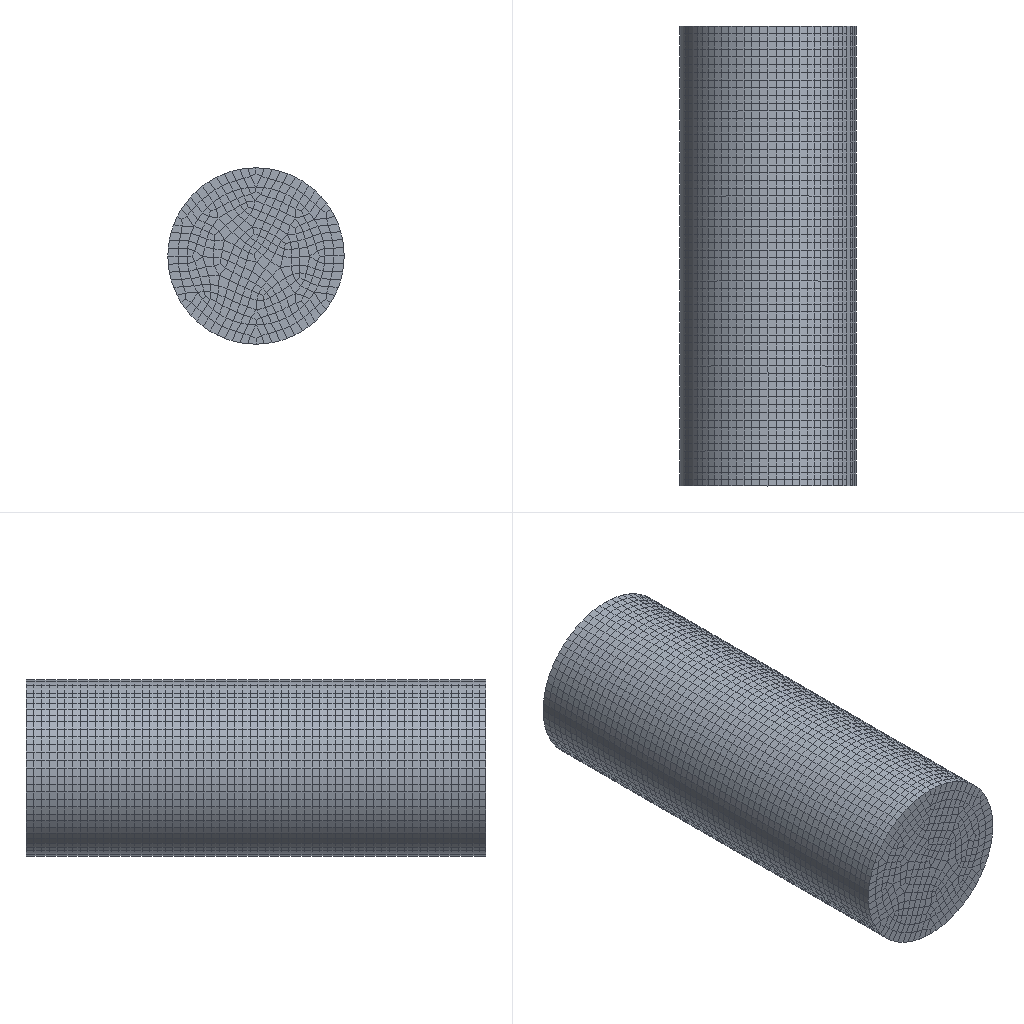Simulation study | ansys workbench
Ansys APDL input file, long lists of numbers shortened:
/batch
/config,noeldb,1     ! force off writing results to database
*get,_wallstrt,active,,time,wall
! ANSYS input file written by Workbench version 2020 R2
! File used for geometry attach:
/title,unsaved_project--___ (B5)
*DIM,_wb_ProjectScratch_dir,string,248
_wb_ProjectScratch_dir(1) = ''
*DIM,_wb_SolverFiles_dir,string,248
_wb_SolverFiles_dir(1) = ''
*DIM,_wb_userfiles_dir,string,248
_wb_userfiles_dir(1) = ''
/com,--- Data in consistent MKS units. See Solving Units in the help system for more information.
/units,MKS
/nopr
/wb,file,start              !  signify a WB generated input file
/prep7
! Turn off shape checking because checks already performed inside WB mesher.
! See help system for more information.
SHPP,OFF,,NOWARN
/nolist
etcon,set             ! allow ANSYS to choose best KEYOP's for 180x elements
/com,*********** Nodes for the whole assembly ***********
nblock,3,,50740
(1i9,3e20.9e3)
        1    -1.192148224E-02     0.000000000E+00    -1.104059469E-02
! (46127 more lines like these left out)
-1
/wb,elem,start            !  set before creation of elements
/com,*********** Elements for Body 1 "SYS\__" ***********
et,1,90
eblock,19,solid,,8511
(19i9)
        1        1        1        1        0        0        0        0       20        0        1      424      532    12288    12285      422      531    12424    12421
! (17021 more lines like these left out)
-1
/wb,elem,end               !  done creating elements
/com,*********** Send User Defined Coordinate System(s) ***********
csys,0
toffst,273.15,  ! Temperature offset from absolute zero
/wb,mat,start              !  starting to send materials
/com,*********** Send Materials ***********
Temperature = 'TEMP' ! Temperature
MP,DENS,1,7850,	! kg m^-3
MP,ALPX,1,1.2e-05,	! C^-1
MP,C,1,434,	! J kg^-1 C^-1
MP,KXX,1,60.5,	! W m^-1 C^-1
MP,RSVX,1,1.7e-07,	! kg m^3 A^-2 s^-3
MP,EX,1,200000000000,	! Pa
MP,NUXY,1,0.3,
MP,MURX,1,10000,
/wb,mat,end                !  done sending materials
!************************* Model Summary ********************
!SYS\__,	Structural Steel,	matid,	1
!************************* End Model Summary ********************
! get the diagonal of the bounding box. Needed later for other things
*get,_xmin,node,,mnloc,x
*get,_ymin,node,,mnloc,y
*get,_zmin,node,,mnloc,z
*get,_xmax,node,,mxloc,x
*get,_ymax,node,,mxloc,y
*get,_zmax,node,,mxloc,z
_ASMDIAG=(_xmax-_xmin)*(_xmax-_xmin)+(_ymax-_ymin)*(_ymax-_ymin)+(_zmax-_zmin)*(_zmax-_zmin)
_ASMDIAG=SQRT(_ASMDIAG)
/wb,contact,start          !  starting to send contact
/wb,contact,end            !  done creating contacts
/golist
/wb,load,start             !  starting to send loads
/com,*********** Define Temperature Constraint ***********
CMBLOCK,_CM52   ,NODE,    10344
(8i10)
       799       800       801       802       803       804       805       806
! (1292 more lines like these left out)
*DIM,_loadvari52,TABLE,2,1,1,TIME,
! Time values
_loadvari52(1,0,1) = 0.
_loadvari52(2,0,1) = 1.
! Load values
_loadvari52(1,1,1) = 100.
_loadvari52(2,1,1) = 100.
fcum,add                   ! add nodal forces up (needed in case have loads on the same edge,vertex)
fcum                       ! reset default on fcum command since done sending WB F loads
/com,*********** Create "______" ***********
et,2,152
eblock,10,,,4080
(15i9)
    16518        2        2        2        0    12215    12217    12081    12079    45179    45178    44727    45173
! (4079 more lines like these left out)
-1
esel,s,type,,2
keyop,2,8,2.
keyop,2,13,0
esel,all
/com,***************** Define Uniform Initial temperature ***************
tunif,22.
/gst,on,on
fini
*get,_numnode,node,0,count
*get,_numelem,elem,0,count
*get, _MAXELEMNUM, elem, 0, NUM, MAX
*get, _MAXNODENUM, node, 0, NUM, MAX
*get, _MAXELEMTYPE, etyp, 0, NUM, MAX
*get, _MAXREALCONST, real, 0, NUM, MAX
/go
/wb,load,end               !  done creating loads
/com,--- Number of total nodes = %_numnode%
/com,--- Number of contact elements = 4080
/com,--- Number of spring elements = 0
/com,--- Number of bearing elements = 0
/com,--- Number of solid elements = 8511
/com,--- Number of condensed parts = 0
/com,--- Number of total elements = %_numelem%
*get,_wallbsol,active,,time,wall
/com,****************************************************************************
/com,*************************    SOLUTION       ********************************
/com,****************************************************************************
/solu
antype,4                   ! transient analysis
kbc,1                      ! stepped BC's
!eqsl,sparse               ! using sparse solver which is default so no eqsl command needed
cntr,print,1               ! print out contact info and also make no initial contact an error
rescontrol,,none                 ! Do not keep any restart files
thopt,quasi,5.e-002
nlhist,nsol,MAX_TEMP,temp,max
nlhist,nsol,MIN_TEMP,temp,min
/com,********* Initial Time Increment Check And Fourier Modulus *********
/com, Specified Initial Time Increment: 0.1
/com, Estimated Increment Needed, le*le/alpha, Body 1: 0.2533
/com,****************************************************
/com,******************* SOLVE FOR LS 1 OF 1 ****************
d,_CM52,temp,%_loadvari52%
esel,s,type,,2
nsle
sf,all,conv,250.,22.
nsel,all
esel,all
autots,on
nsub,100,1000,10
time,10.
timint,on                  ! Turn on time integration effects
outres,erase
outres,all,none
outres,nsol,all
outres,rsol,all
outres,eangl,all
outres,veng,all
outres,fflux,all
outres,cont,all
/nopr
esel,s,type,,2
cm,_elmisc,elem
esel,all
/gopr
outres,misc,all,_elmisc
cnvtol,heat,,.001,,1.e-006    ! Program Controlled. Set MINREF equivalent of 1e-6 Watts
! *********** WB SOLVE COMMAND ***********
! check interactive state
*get,ANSINTER_,active,,int
*if,ANSINTER_,ne,0,then
/eof
*endif
solve
/com *************** Write FE CONNECTORS *********
CEWRITE,file,ce,,INTE
/com,****************************************************
/com,*************** FINISHED SOLVE FOR LS 1 *************
*get,_wallasol,active,,time,wall
/post1
xmlo,ENCODING,ISO-8859-1
xmlo,parm
/xml,parm,xml
fini
/gopr
*get,_walldone,active,,time,wall
_preptime=(_wallbsol-_wallstrt)*3600
_solvtime=(_wallasol-_wallbsol)*3600
_posttime=(_walldone-_wallasol)*3600
_totaltim=(_walldone-_wallstrt)*3600
*get,_dlbratio,active,0,solu,dlbr
*get,_combtime,active,0,solu,comb
/com,--- Total number of nodes = %_numnode%
/com,--- Total number of elements = %_numelem%
/com,--- Element load balance ratio = %_dlbratio%
/com,--- Time to combine distributed files = %_combtime%
/wb,file,end               ! done with WB generated input